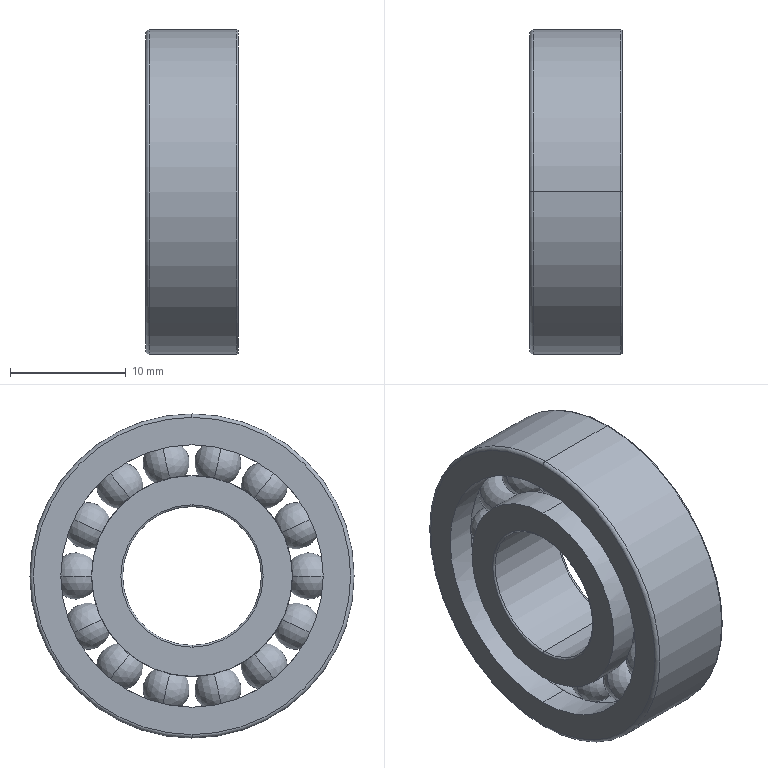Part | NX | 1 solid | 100 faces | box 8 x 28 x 28 mm | volume 2885 mm3 | torus 53 | sphere 28 | cylinder 14 | plane 5 | commonest cylinder face diameters 17.333 x4 12 x2 22.667 x2 23.347 x2 24.547 x2 28 x2